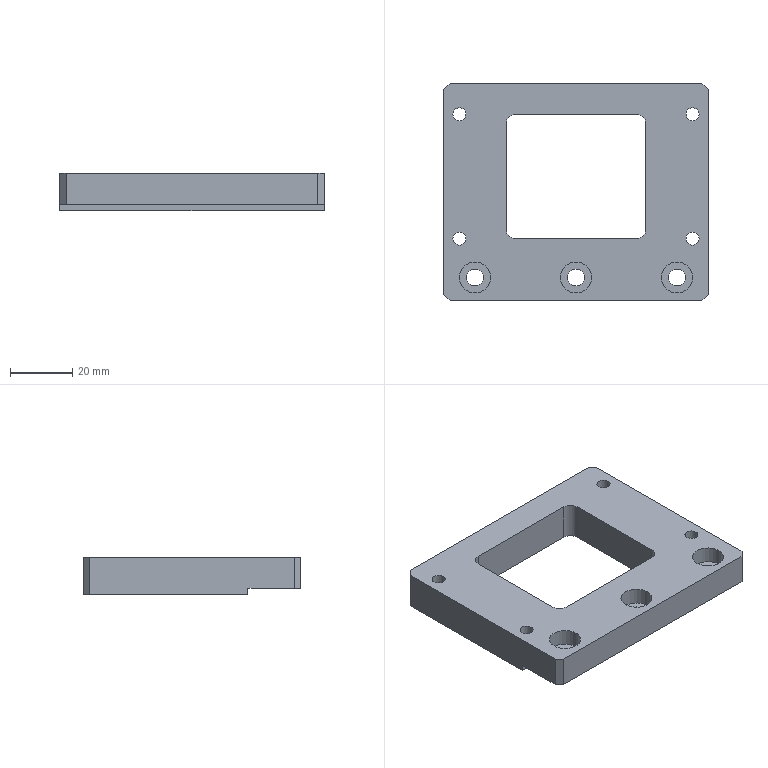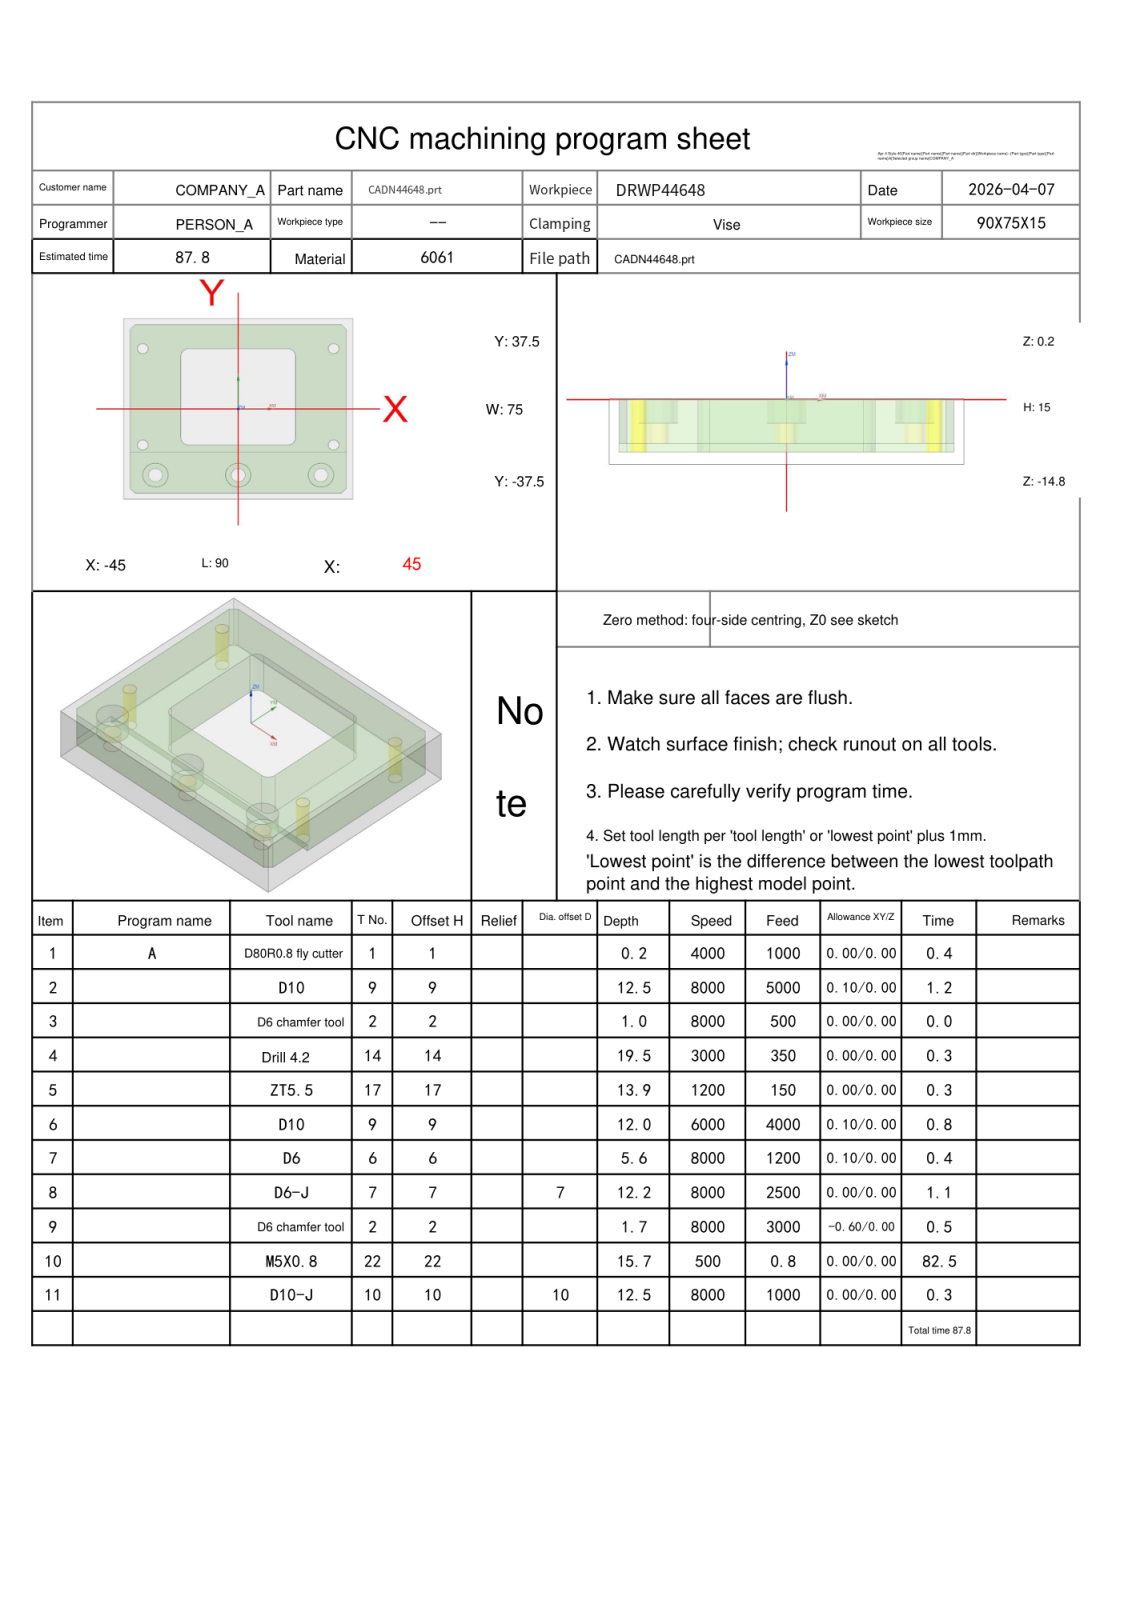NC program | NX | posted by the shop | part box 85 x 70 x 12 mm
Lines 580 to 1629 of 5800:
N8 T07 M06
(D6-J  D=6. R=0. H=07 ce=0.00 di=0.00)
G00 G90 G54 X32.5 Y-27.5 M03 S8000
G43 H07 Z20.
M08
Z0.0
G41 D07
G01 X32.54 Y-27.696 F500.
G03 X33.51 Y-28.49 I.97 J.196
X34.5 Y-27.5 I0.0 J.99
X34.5 Y-27.5 Z-5. I-2. J0.0
X34.253 Y-26.536 Z-5.4 I-2. J0.0
X32.5 Y-25.5 I-1.753 J-.964
X30.5 Y-27.5 I0.0 J-2.
X32.5 Y-29.5 I2. J0.0
X34.5 Y-27.5 I0.0 J2.
X34.253 Y-26.536 I-2. J0.0
X33.385 Y-26.023 I-.868 J-.477
X32.395 Y-27.013 I0.0 J-.99
X32.44 Y-27.309 I.99 J0.0
G01 G40 X32.5 Y-27.5
G00 Z20.
X0.0
Z0.0
G41 D07
G01 X.04 Y-27.696
G03 X1.01 Y-28.49 I.97 J.196
X2. Y-27.5 I0.0 J.99
X2. Y-27.5 Z-5. I-2. J0.0
X1.753 Y-26.536 Z-5.4 I-2. J0.0
X0.0 Y-25.5 I-1.753 J-.964
X-2. Y-27.5 I0.0 J-2.
X0.0 Y-29.5 I2. J0.0
X2. Y-27.5 I0.0 J2.
X1.753 Y-26.536 I-2. J0.0
X.885 Y-26.023 I-.868 J-.477
X-.105 Y-27.013 I0.0 J-.99
X-.06 Y-27.309 I.99 J0.0
G01 G40 X0.0 Y-27.5
G00 Z20.
X-32.5
Z0.0
G41 D07
G01 X-32.46 Y-27.696
G03 X-31.49 Y-28.49 I.97 J.196
X-30.5 Y-27.5 I0.0 J.99
X-30.5 Y-27.5 Z-5. I-2. J0.0
X-30.747 Y-26.536 Z-5.4 I-2. J0.0
X-32.5 Y-25.5 I-1.753 J-.964
X-34.5 Y-27.5 I0.0 J-2.
X-32.5 Y-29.5 I2. J0.0
X-30.5 Y-27.5 I0.0 J2.
X-30.747 Y-26.536 I-2. J0.0
X-31.615 Y-26.023 I-.868 J-.477
X-32.605 Y-27.013 I0.0 J-.99
X-32.56 Y-27.309 I.99 J0.0
G01 G40 X-32.5 Y-27.5
G00 Z20.
G00 G90 X16.684 Y-11.1 M03 S6000
Z20.
Z.6
G01 X16.685 Y-11.11 Z.471 F2000.
X16.69 Y-11.139 Z.355
X16.698 Y-11.183 Z.25
X16.71 Y-11.241 Z.156
X16.726 Y-11.309 Z.072
X16.747 Y-11.385 Z-.001
X16.773 Y-11.466 Z-.065
X16.804 Y-11.55 Z-.12
X16.84 Y-11.634 Z-.166
X16.883 Y-11.715 Z-.205
X16.932 Y-11.791 Z-.236
X16.987 Y-11.859 Z-.261
X17.05 Y-11.917 Z-.279
X17.12 Y-11.961 Z-.291
X17.198 Y-11.99 Z-.298
X17.284 Y-12. Z-.3
X19.5 F2500.
Y-9.784
X19.484 Y-9.711 Z-.301
X19.437 Y-9.657 Z-.304
X19.364 Y-9.619 Z-.308
X19.269 Y-9.598 Z-.313
X19.155 Y-9.59 Z-.32
X19.026 Y-9.596 Z-.328
X18.888 Y-9.613 Z-.338
X18.742 Y-9.642 Z-.347
X18.594 Y-9.679 Z-.358
X18.447 Y-9.725 Z-.369
X18.306 Y-9.778 Z-.381
X18.069 Y-9.89 Z-.404
X17.861 Y-10.023 Z-.427
X17.679 Y-10.179 Z-.45
X17.523 Y-10.361 Z-.473
X17.39 Y-10.569 Z-.496
X17.278 Y-10.806 Z-.519
X17.225 Y-10.947 Z-.531
X17.179 Y-11.094 Z-.542
X17.142 Y-11.242 Z-.553
X17.113 Y-11.388 Z-.562
X17.096 Y-11.526 Z-.572
X17.09 Y-11.655 Z-.58
X17.098 Y-11.769 Z-.587
X17.119 Y-11.864 Z-.592
X17.157 Y-11.937 Z-.596
X17.211 Y-11.984 Z-.599
X17.284 Y-12. Z-.6
X19.5
Y-9.784
X19.484 Y-9.711 Z-.601
X19.437 Y-9.657 Z-.604
X19.364 Y-9.619 Z-.608
X19.269 Y-9.598 Z-.613
X19.155 Y-9.59 Z-.62
X19.026 Y-9.596 Z-.628
X18.888 Y-9.613 Z-.638
X18.742 Y-9.642 Z-.647
X18.594 Y-9.679 Z-.658
X18.447 Y-9.725 Z-.669
X18.306 Y-9.778 Z-.681
X18.069 Y-9.89 Z-.704
X17.861 Y-10.023 Z-.727
X17.679 Y-10.179 Z-.75
X17.523 Y-10.361 Z-.773
X17.39 Y-10.569 Z-.796
X17.278 Y-10.806 Z-.819
X17.225 Y-10.947 Z-.831
X17.179 Y-11.094 Z-.842
X17.142 Y-11.242 Z-.853
X17.113 Y-11.388 Z-.862
X17.096 Y-11.526 Z-.872
X17.09 Y-11.655 Z-.88
X17.098 Y-11.769 Z-.887
X17.119 Y-11.864 Z-.892
X17.157 Y-11.937 Z-.896
X17.211 Y-11.984 Z-.899
X17.284 Y-12. Z-.9
X19.5
Y-9.784
X19.484 Y-9.711 Z-.901
X19.437 Y-9.657 Z-.904
X19.364 Y-9.619 Z-.908
X19.269 Y-9.598 Z-.913
X19.155 Y-9.59 Z-.92
X19.026 Y-9.596 Z-.928
X18.888 Y-9.613 Z-.938
X18.742 Y-9.642 Z-.947
X18.594 Y-9.679 Z-.958
X18.447 Y-9.725 Z-.969
X18.306 Y-9.778 Z-.981
X18.069 Y-9.89 Z-1.004
X17.861 Y-10.023 Z-1.027
X17.679 Y-10.179 Z-1.05
X17.523 Y-10.361 Z-1.073
X17.39 Y-10.569 Z-1.096
X17.278 Y-10.806 Z-1.119
X17.225 Y-10.947 Z-1.131
X17.179 Y-11.094 Z-1.142
X17.142 Y-11.242 Z-1.153
X17.113 Y-11.388 Z-1.162
X17.096 Y-11.526 Z-1.172
X17.09 Y-11.655 Z-1.18
X17.098 Y-11.769 Z-1.187
X17.119 Y-11.864 Z-1.192
X17.157 Y-11.937 Z-1.196
X17.211 Y-11.984 Z-1.199
X17.284 Y-12. Z-1.2
X19.5
Y-9.784
X19.484 Y-9.711 Z-1.201
X19.437 Y-9.657 Z-1.204
X19.364 Y-9.619 Z-1.208
X19.269 Y-9.598 Z-1.213
X19.155 Y-9.59 Z-1.22
X19.026 Y-9.596 Z-1.228
X18.888 Y-9.613 Z-1.238
X18.742 Y-9.642 Z-1.247
X18.594 Y-9.679 Z-1.258
X18.447 Y-9.725 Z-1.269
X18.306 Y-9.778 Z-1.281
X18.069 Y-9.89 Z-1.304
X17.861 Y-10.023 Z-1.327
X17.679 Y-10.179 Z-1.35
X17.523 Y-10.361 Z-1.373
X17.39 Y-10.569 Z-1.396
X17.278 Y-10.806 Z-1.419
X17.225 Y-10.947 Z-1.431
X17.179 Y-11.094 Z-1.442
X17.142 Y-11.242 Z-1.453
X17.113 Y-11.388 Z-1.462
X17.096 Y-11.526 Z-1.472
X17.09 Y-11.655 Z-1.48
X17.098 Y-11.769 Z-1.487
X17.119 Y-11.864 Z-1.492
X17.157 Y-11.937 Z-1.496
X17.211 Y-11.984 Z-1.499
X17.284 Y-12. Z-1.5
X19.5
Y-9.784
X19.484 Y-9.711 Z-1.501
X19.437 Y-9.657 Z-1.504
X19.364 Y-9.619 Z-1.508
X19.269 Y-9.598 Z-1.513
X19.155 Y-9.59 Z-1.52
X19.026 Y-9.596 Z-1.528
X18.888 Y-9.613 Z-1.538
X18.742 Y-9.642 Z-1.547
X18.594 Y-9.679 Z-1.558
X18.447 Y-9.725 Z-1.569
X18.306 Y-9.778 Z-1.581
X18.069 Y-9.89 Z-1.604
X17.861 Y-10.023 Z-1.627
X17.679 Y-10.179 Z-1.65
X17.523 Y-10.361 Z-1.673
X17.39 Y-10.569 Z-1.696
X17.278 Y-10.806 Z-1.719
X17.225 Y-10.947 Z-1.731
X17.179 Y-11.094 Z-1.742
X17.142 Y-11.242 Z-1.753
X17.113 Y-11.388 Z-1.762
X17.096 Y-11.526 Z-1.772
X17.09 Y-11.655 Z-1.78
X17.098 Y-11.769 Z-1.787
X17.119 Y-11.864 Z-1.792
X17.157 Y-11.937 Z-1.796
X17.211 Y-11.984 Z-1.799
X17.284 Y-12. Z-1.8
X19.5
Y-9.784
X19.484 Y-9.711 Z-1.801
X19.437 Y-9.657 Z-1.804
X19.364 Y-9.619 Z-1.808
X19.269 Y-9.598 Z-1.813
X19.155 Y-9.59 Z-1.82
X19.026 Y-9.596 Z-1.828
X18.888 Y-9.613 Z-1.838
X18.742 Y-9.642 Z-1.847
X18.594 Y-9.679 Z-1.858
X18.447 Y-9.725 Z-1.869
X18.306 Y-9.778 Z-1.881
X18.069 Y-9.89 Z-1.904
X17.861 Y-10.023 Z-1.927
X17.679 Y-10.179 Z-1.95
X17.523 Y-10.361 Z-1.973
X17.39 Y-10.569 Z-1.996
X17.278 Y-10.806 Z-2.019
X17.225 Y-10.947 Z-2.031
X17.179 Y-11.094 Z-2.042
X17.142 Y-11.242 Z-2.053
X17.113 Y-11.388 Z-2.062
X17.096 Y-11.526 Z-2.072
X17.09 Y-11.655 Z-2.08
X17.098 Y-11.769 Z-2.087
X17.119 Y-11.864 Z-2.092
X17.157 Y-11.937 Z-2.096
X17.211 Y-11.984 Z-2.099
X17.284 Y-12. Z-2.1
X19.5
Y-9.784
X19.484 Y-9.711 Z-2.101
X19.437 Y-9.657 Z-2.104
X19.364 Y-9.619 Z-2.108
X19.269 Y-9.598 Z-2.113
X19.155 Y-9.59 Z-2.12
X19.026 Y-9.596 Z-2.128
X18.888 Y-9.613 Z-2.138
X18.742 Y-9.642 Z-2.147
X18.594 Y-9.679 Z-2.158
X18.447 Y-9.725 Z-2.169
X18.306 Y-9.778 Z-2.181
X18.069 Y-9.89 Z-2.204
X17.861 Y-10.023 Z-2.227
X17.679 Y-10.179 Z-2.25
X17.523 Y-10.361 Z-2.273
X17.39 Y-10.569 Z-2.296
X17.278 Y-10.806 Z-2.319
X17.225 Y-10.947 Z-2.331
X17.179 Y-11.094 Z-2.342
X17.142 Y-11.242 Z-2.353
X17.113 Y-11.388 Z-2.362
X17.096 Y-11.526 Z-2.372
X17.09 Y-11.655 Z-2.38
X17.098 Y-11.769 Z-2.387
X17.119 Y-11.864 Z-2.392
X17.157 Y-11.937 Z-2.396
X17.211 Y-11.984 Z-2.399
X17.284 Y-12. Z-2.4
X19.5
Y-9.784
X19.484 Y-9.711 Z-2.401
X19.437 Y-9.657 Z-2.404
X19.364 Y-9.619 Z-2.408
X19.269 Y-9.598 Z-2.413
X19.155 Y-9.59 Z-2.42
X19.026 Y-9.596 Z-2.428
X18.888 Y-9.613 Z-2.438
X18.742 Y-9.642 Z-2.447
X18.594 Y-9.679 Z-2.458
X18.447 Y-9.725 Z-2.469
X18.306 Y-9.778 Z-2.481
X18.069 Y-9.89 Z-2.504
X17.861 Y-10.023 Z-2.527
X17.679 Y-10.179 Z-2.55
X17.523 Y-10.361 Z-2.573
X17.39 Y-10.569 Z-2.596
X17.278 Y-10.806 Z-2.619
X17.225 Y-10.947 Z-2.631
X17.179 Y-11.094 Z-2.642
X17.142 Y-11.242 Z-2.653
X17.113 Y-11.388 Z-2.662
X17.096 Y-11.526 Z-2.672
X17.09 Y-11.655 Z-2.68
X17.098 Y-11.769 Z-2.687
X17.119 Y-11.864 Z-2.692
X17.157 Y-11.937 Z-2.696
X17.211 Y-11.984 Z-2.699
X17.284 Y-12. Z-2.7
X19.5
Y-9.784
X19.484 Y-9.711 Z-2.701
X19.437 Y-9.657 Z-2.704
X19.364 Y-9.619 Z-2.708
X19.269 Y-9.598 Z-2.713
X19.155 Y-9.59 Z-2.72
X19.026 Y-9.596 Z-2.728
X18.888 Y-9.613 Z-2.738
X18.742 Y-9.642 Z-2.747
X18.594 Y-9.679 Z-2.758
X18.447 Y-9.725 Z-2.769
X18.306 Y-9.778 Z-2.781
X18.069 Y-9.89 Z-2.804
X17.861 Y-10.023 Z-2.827
X17.679 Y-10.179 Z-2.85
X17.523 Y-10.361 Z-2.873
X17.39 Y-10.569 Z-2.896
X17.278 Y-10.806 Z-2.919
X17.225 Y-10.947 Z-2.931
X17.179 Y-11.094 Z-2.942
X17.142 Y-11.242 Z-2.953
X17.113 Y-11.388 Z-2.962
X17.096 Y-11.526 Z-2.972
X17.09 Y-11.655 Z-2.98
X17.098 Y-11.769 Z-2.987
X17.119 Y-11.864 Z-2.992
X17.157 Y-11.937 Z-2.996
X17.211 Y-11.984 Z-2.999
X17.284 Y-12. Z-3.
X19.5
Y-9.784
X19.484 Y-9.711 Z-3.001
X19.437 Y-9.657 Z-3.004
X19.364 Y-9.619 Z-3.008
X19.269 Y-9.598 Z-3.013
X19.155 Y-9.59 Z-3.02
X19.026 Y-9.596 Z-3.028
X18.888 Y-9.613 Z-3.038
X18.742 Y-9.642 Z-3.047
X18.594 Y-9.679 Z-3.058
X18.447 Y-9.725 Z-3.069
X18.306 Y-9.778 Z-3.081
X18.069 Y-9.89 Z-3.104
X17.861 Y-10.023 Z-3.127
X17.679 Y-10.179 Z-3.15
X17.523 Y-10.361 Z-3.173
X17.39 Y-10.569 Z-3.196
X17.278 Y-10.806 Z-3.219
X17.225 Y-10.947 Z-3.231
X17.179 Y-11.094 Z-3.242
X17.142 Y-11.242 Z-3.253
X17.113 Y-11.388 Z-3.262
X17.096 Y-11.526 Z-3.272
X17.09 Y-11.655 Z-3.28
X17.098 Y-11.769 Z-3.287
X17.119 Y-11.864 Z-3.292
X17.157 Y-11.937 Z-3.296
X17.211 Y-11.984 Z-3.299
X17.284 Y-12. Z-3.3
X19.5
Y-9.784
X19.484 Y-9.711 Z-3.301
X19.437 Y-9.657 Z-3.304
X19.364 Y-9.619 Z-3.308
X19.269 Y-9.598 Z-3.313
X19.155 Y-9.59 Z-3.32
X19.026 Y-9.596 Z-3.328
X18.888 Y-9.613 Z-3.338
X18.742 Y-9.642 Z-3.347
X18.594 Y-9.679 Z-3.358
X18.447 Y-9.725 Z-3.369
X18.306 Y-9.778 Z-3.381
X18.069 Y-9.89 Z-3.404
X17.861 Y-10.023 Z-3.427
X17.679 Y-10.179 Z-3.45
X17.523 Y-10.361 Z-3.473
X17.39 Y-10.569 Z-3.496
X17.278 Y-10.806 Z-3.519
X17.225 Y-10.947 Z-3.531
X17.179 Y-11.094 Z-3.542
X17.142 Y-11.242 Z-3.553
X17.113 Y-11.388 Z-3.562
X17.096 Y-11.526 Z-3.572
X17.09 Y-11.655 Z-3.58
X17.098 Y-11.769 Z-3.587
X17.119 Y-11.864 Z-3.592
X17.157 Y-11.937 Z-3.596
X17.211 Y-11.984 Z-3.599
X17.284 Y-12. Z-3.6
X19.5
Y-9.784
X19.484 Y-9.711 Z-3.601
X19.437 Y-9.657 Z-3.604
X19.364 Y-9.619 Z-3.608
X19.269 Y-9.598 Z-3.613
X19.155 Y-9.59 Z-3.62
X19.026 Y-9.596 Z-3.628
X18.888 Y-9.613 Z-3.638
X18.742 Y-9.642 Z-3.647
X18.594 Y-9.679 Z-3.658
X18.447 Y-9.725 Z-3.669
X18.306 Y-9.778 Z-3.681
X18.069 Y-9.89 Z-3.704
X17.861 Y-10.023 Z-3.727
X17.679 Y-10.179 Z-3.75
X17.523 Y-10.361 Z-3.773
X17.39 Y-10.569 Z-3.796
X17.278 Y-10.806 Z-3.819
X17.225 Y-10.947 Z-3.831
X17.179 Y-11.094 Z-3.842
X17.142 Y-11.242 Z-3.853
X17.113 Y-11.388 Z-3.862
X17.096 Y-11.526 Z-3.872
X17.09 Y-11.655 Z-3.88
X17.098 Y-11.769 Z-3.887
X17.119 Y-11.864 Z-3.892
X17.157 Y-11.937 Z-3.896
X17.211 Y-11.984 Z-3.899
X17.284 Y-12. Z-3.9
X19.5
Y-9.784
X19.484 Y-9.711 Z-3.901
X19.437 Y-9.657 Z-3.904
X19.364 Y-9.619 Z-3.908
X19.269 Y-9.598 Z-3.913
X19.155 Y-9.59 Z-3.92
X19.026 Y-9.596 Z-3.928
X18.888 Y-9.613 Z-3.938
X18.742 Y-9.642 Z-3.947
X18.594 Y-9.679 Z-3.958
X18.447 Y-9.725 Z-3.969
X18.306 Y-9.778 Z-3.981
X18.069 Y-9.89 Z-4.004
X17.861 Y-10.023 Z-4.027
X17.679 Y-10.179 Z-4.05
X17.523 Y-10.361 Z-4.073
X17.39 Y-10.569 Z-4.096
X17.278 Y-10.806 Z-4.119
X17.225 Y-10.947 Z-4.131
X17.179 Y-11.094 Z-4.142
X17.142 Y-11.242 Z-4.153
X17.113 Y-11.388 Z-4.162
X17.096 Y-11.526 Z-4.172
X17.09 Y-11.655 Z-4.18
X17.098 Y-11.769 Z-4.187
X17.119 Y-11.864 Z-4.192
X17.157 Y-11.937 Z-4.196
X17.211 Y-11.984 Z-4.199
X17.284 Y-12. Z-4.2
X19.5
Y-9.784
X19.484 Y-9.711 Z-4.201
X19.437 Y-9.657 Z-4.204
X19.364 Y-9.619 Z-4.208
X19.269 Y-9.598 Z-4.213
X19.155 Y-9.59 Z-4.22
X19.026 Y-9.596 Z-4.228
X18.888 Y-9.613 Z-4.238
X18.742 Y-9.642 Z-4.247
X18.594 Y-9.679 Z-4.258
X18.447 Y-9.725 Z-4.269
X18.306 Y-9.778 Z-4.281
X18.069 Y-9.89 Z-4.304
X17.861 Y-10.023 Z-4.327
X17.679 Y-10.179 Z-4.35
X17.523 Y-10.361 Z-4.373
X17.39 Y-10.569 Z-4.396
X17.278 Y-10.806 Z-4.419
X17.225 Y-10.947 Z-4.431
X17.179 Y-11.094 Z-4.442
X17.142 Y-11.242 Z-4.453
X17.113 Y-11.388 Z-4.462
X17.096 Y-11.526 Z-4.472
X17.09 Y-11.655 Z-4.48
X17.098 Y-11.769 Z-4.487
X17.119 Y-11.864 Z-4.492
X17.157 Y-11.937 Z-4.496
X17.211 Y-11.984 Z-4.499
X17.284 Y-12. Z-4.5
X19.5
Y-9.784
X19.484 Y-9.711 Z-4.501
X19.437 Y-9.657 Z-4.504
X19.364 Y-9.619 Z-4.508
X19.269 Y-9.598 Z-4.513
X19.155 Y-9.59 Z-4.52
X19.026 Y-9.596 Z-4.528
X18.888 Y-9.613 Z-4.538
X18.742 Y-9.642 Z-4.547
X18.594 Y-9.679 Z-4.558
X18.447 Y-9.725 Z-4.569
X18.306 Y-9.778 Z-4.581
X18.069 Y-9.89 Z-4.604
X17.861 Y-10.023 Z-4.627
X17.679 Y-10.179 Z-4.65
X17.523 Y-10.361 Z-4.673
X17.39 Y-10.569 Z-4.696
X17.278 Y-10.806 Z-4.719
X17.225 Y-10.947 Z-4.731
X17.179 Y-11.094 Z-4.742
X17.142 Y-11.242 Z-4.753
X17.113 Y-11.388 Z-4.762
X17.096 Y-11.526 Z-4.772
X17.09 Y-11.655 Z-4.78
X17.098 Y-11.769 Z-4.787
X17.119 Y-11.864 Z-4.792
X17.157 Y-11.937 Z-4.796
X17.211 Y-11.984 Z-4.799
X17.284 Y-12. Z-4.8
X19.5
Y-9.784
X19.484 Y-9.711 Z-4.801
X19.437 Y-9.657 Z-4.804
X19.364 Y-9.619 Z-4.808
X19.269 Y-9.598 Z-4.813
X19.155 Y-9.59 Z-4.82
X19.026 Y-9.596 Z-4.828
X18.888 Y-9.613 Z-4.838
X18.742 Y-9.642 Z-4.847
X18.594 Y-9.679 Z-4.858
X18.447 Y-9.725 Z-4.869
X18.306 Y-9.778 Z-4.881
X18.069 Y-9.89 Z-4.904
X17.861 Y-10.023 Z-4.927
X17.679 Y-10.179 Z-4.95
X17.523 Y-10.361 Z-4.973
X17.39 Y-10.569 Z-4.996
X17.278 Y-10.806 Z-5.019
X17.225 Y-10.947 Z-5.031
X17.179 Y-11.094 Z-5.042
X17.142 Y-11.242 Z-5.053
X17.113 Y-11.388 Z-5.062
X17.096 Y-11.526 Z-5.072
X17.09 Y-11.655 Z-5.08
X17.098 Y-11.769 Z-5.087
X17.119 Y-11.864 Z-5.092
X17.157 Y-11.937 Z-5.096
X17.211 Y-11.984 Z-5.099
X17.284 Y-12. Z-5.1
X19.5
Y-9.784
X19.484 Y-9.711 Z-5.101
X19.437 Y-9.657 Z-5.104
X19.364 Y-9.619 Z-5.108
X19.269 Y-9.598 Z-5.113
X19.155 Y-9.59 Z-5.12
X19.026 Y-9.596 Z-5.128
X18.888 Y-9.613 Z-5.138
X18.742 Y-9.642 Z-5.147
X18.594 Y-9.679 Z-5.158
X18.447 Y-9.725 Z-5.169
X18.306 Y-9.778 Z-5.181
X18.069 Y-9.89 Z-5.204
X17.861 Y-10.023 Z-5.227
X17.679 Y-10.179 Z-5.25
X17.523 Y-10.361 Z-5.273
X17.39 Y-10.569 Z-5.296
X17.278 Y-10.806 Z-5.319
X17.225 Y-10.947 Z-5.331
X17.179 Y-11.094 Z-5.342
X17.142 Y-11.242 Z-5.353
X17.113 Y-11.388 Z-5.362
X17.096 Y-11.526 Z-5.372
X17.09 Y-11.655 Z-5.38
X17.098 Y-11.769 Z-5.387
X17.119 Y-11.864 Z-5.392
X17.157 Y-11.937 Z-5.396
X17.211 Y-11.984 Z-5.399
X17.284 Y-12. Z-5.4
X19.5
Y-9.784
X19.484 Y-9.711 Z-5.401
X19.437 Y-9.657 Z-5.404
X19.364 Y-9.619 Z-5.408
X19.269 Y-9.598 Z-5.413
X19.155 Y-9.59 Z-5.42
X19.026 Y-9.596 Z-5.428
X18.888 Y-9.613 Z-5.438
X18.742 Y-9.642 Z-5.447
X18.594 Y-9.679 Z-5.458
X18.447 Y-9.725 Z-5.469
X18.306 Y-9.778 Z-5.481
X18.069 Y-9.89 Z-5.504
X17.861 Y-10.023 Z-5.527
X17.679 Y-10.179 Z-5.55
X17.523 Y-10.361 Z-5.573
X17.39 Y-10.569 Z-5.596
X17.278 Y-10.806 Z-5.619
X17.225 Y-10.947 Z-5.631
X17.179 Y-11.094 Z-5.642
X17.142 Y-11.242 Z-5.653
X17.113 Y-11.388 Z-5.662
X17.096 Y-11.526 Z-5.672
X17.09 Y-11.655 Z-5.68
X17.098 Y-11.769 Z-5.687
X17.119 Y-11.864 Z-5.692
X17.157 Y-11.937 Z-5.696
X17.211 Y-11.984 Z-5.699
X17.284 Y-12. Z-5.7
X19.5
Y-9.784
X19.484 Y-9.711 Z-5.701
X19.437 Y-9.657 Z-5.704
X19.364 Y-9.619 Z-5.708
X19.269 Y-9.598 Z-5.713
X19.155 Y-9.59 Z-5.72
X19.026 Y-9.596 Z-5.728
X18.888 Y-9.613 Z-5.738
X18.742 Y-9.642 Z-5.747
X18.594 Y-9.679 Z-5.758
X18.447 Y-9.725 Z-5.769
X18.306 Y-9.778 Z-5.781
X18.069 Y-9.89 Z-5.804
X17.861 Y-10.023 Z-5.827
X17.679 Y-10.179 Z-5.85
X17.523 Y-10.361 Z-5.873
X17.39 Y-10.569 Z-5.896
X17.278 Y-10.806 Z-5.919
X17.225 Y-10.947 Z-5.931
X17.179 Y-11.094 Z-5.942
X17.142 Y-11.242 Z-5.953
X17.113 Y-11.388 Z-5.962
X17.096 Y-11.526 Z-5.972
X17.09 Y-11.655 Z-5.98
X17.098 Y-11.769 Z-5.987
X17.119 Y-11.864 Z-5.992
X17.157 Y-11.937 Z-5.996
X17.211 Y-11.984 Z-5.999
X17.284 Y-12. Z-6.
X19.5
Y-9.784
X19.484 Y-9.711 Z-6.001
X19.437 Y-9.657 Z-6.004
X19.364 Y-9.619 Z-6.008
X19.269 Y-9.598 Z-6.013
X19.155 Y-9.59 Z-6.02
X19.026 Y-9.596 Z-6.028
X18.888 Y-9.613 Z-6.038
X18.742 Y-9.642 Z-6.047
X18.594 Y-9.679 Z-6.058
X18.447 Y-9.725 Z-6.069
X18.306 Y-9.778 Z-6.081
X18.069 Y-9.89 Z-6.104
X17.861 Y-10.023 Z-6.127
X17.679 Y-10.179 Z-6.15
X17.523 Y-10.361 Z-6.173
X17.39 Y-10.569 Z-6.196
X17.278 Y-10.806 Z-6.219
X17.225 Y-10.947 Z-6.231
X17.179 Y-11.094 Z-6.242
X17.142 Y-11.242 Z-6.253
X17.113 Y-11.388 Z-6.262
X17.096 Y-11.526 Z-6.272
X17.09 Y-11.655 Z-6.28
X17.098 Y-11.769 Z-6.287
X17.119 Y-11.864 Z-6.292
X17.157 Y-11.937 Z-6.296
X17.211 Y-11.984 Z-6.299
X17.284 Y-12. Z-6.3
X19.5
Y-9.784
X19.484 Y-9.711 Z-6.301
X19.437 Y-9.657 Z-6.304
X19.364 Y-9.619 Z-6.308
X19.269 Y-9.598 Z-6.313
X19.155 Y-9.59 Z-6.32
X19.026 Y-9.596 Z-6.328
X18.888 Y-9.613 Z-6.338
X18.742 Y-9.642 Z-6.347
X18.594 Y-9.679 Z-6.358
X18.447 Y-9.725 Z-6.369
X18.306 Y-9.778 Z-6.381
X18.069 Y-9.89 Z-6.404
X17.861 Y-10.023 Z-6.427
X17.679 Y-10.179 Z-6.45
X17.523 Y-10.361 Z-6.473
X17.39 Y-10.569 Z-6.496
X17.278 Y-10.806 Z-6.519
X17.225 Y-10.947 Z-6.531
X17.179 Y-11.094 Z-6.542
X17.142 Y-11.242 Z-6.553
X17.113 Y-11.388 Z-6.562
X17.096 Y-11.526 Z-6.572
X17.09 Y-11.655 Z-6.58
X17.098 Y-11.769 Z-6.587
X17.119 Y-11.864 Z-6.592
X17.157 Y-11.937 Z-6.596
X17.211 Y-11.984 Z-6.599
X17.284 Y-12. Z-6.6
X19.5
Y-9.784
X19.484 Y-9.711 Z-6.601
X19.437 Y-9.657 Z-6.604
X19.364 Y-9.619 Z-6.608
X19.269 Y-9.598 Z-6.613
X19.155 Y-9.59 Z-6.62
X19.026 Y-9.596 Z-6.628
X18.888 Y-9.613 Z-6.638
X18.742 Y-9.642 Z-6.647
X18.594 Y-9.679 Z-6.658
X18.447 Y-9.725 Z-6.669
X18.306 Y-9.778 Z-6.681
X18.069 Y-9.89 Z-6.704
X17.861 Y-10.023 Z-6.727
X17.679 Y-10.179 Z-6.75
X17.523 Y-10.361 Z-6.773
X17.39 Y-10.569 Z-6.796
X17.278 Y-10.806 Z-6.819
X17.225 Y-10.947 Z-6.831
X17.179 Y-11.094 Z-6.842
X17.142 Y-11.242 Z-6.853
X17.113 Y-11.388 Z-6.862
X17.096 Y-11.526 Z-6.872
X17.09 Y-11.655 Z-6.88
X17.098 Y-11.769 Z-6.887
X17.119 Y-11.864 Z-6.892
X17.157 Y-11.937 Z-6.896
X17.211 Y-11.984 Z-6.899
X17.284 Y-12. Z-6.9
X19.5
Y-9.784
X19.484 Y-9.711 Z-6.901
X19.437 Y-9.657 Z-6.904
X19.364 Y-9.619 Z-6.908
X19.269 Y-9.598 Z-6.913
X19.155 Y-9.59 Z-6.92
X19.026 Y-9.596 Z-6.928
X18.888 Y-9.613 Z-6.938
X18.742 Y-9.642 Z-6.947
X18.594 Y-9.679 Z-6.958
X18.447 Y-9.725 Z-6.969
X18.306 Y-9.778 Z-6.981
X18.069 Y-9.89 Z-7.004
X17.861 Y-10.023 Z-7.027
X17.679 Y-10.179 Z-7.05
X17.523 Y-10.361 Z-7.073
X17.39 Y-10.569 Z-7.096
X17.278 Y-10.806 Z-7.119
X17.225 Y-10.947 Z-7.131
X17.179 Y-11.094 Z-7.142
X17.142 Y-11.242 Z-7.153
X17.113 Y-11.388 Z-7.162
X17.096 Y-11.526 Z-7.172
X17.09 Y-11.655 Z-7.18
X17.098 Y-11.769 Z-7.187
X17.119 Y-11.864 Z-7.192
X17.157 Y-11.937 Z-7.196
X17.211 Y-11.984 Z-7.199
X17.284 Y-12. Z-7.2
X19.5
Y-9.784
X19.484 Y-9.711 Z-7.201
X19.437 Y-9.657 Z-7.204
X19.364 Y-9.619 Z-7.208
X19.269 Y-9.598 Z-7.213
X19.155 Y-9.59 Z-7.22
X19.026 Y-9.596 Z-7.228
X18.888 Y-9.613 Z-7.238
X18.742 Y-9.642 Z-7.247
X18.594 Y-9.679 Z-7.258
X18.447 Y-9.725 Z-7.269
X18.306 Y-9.778 Z-7.281
X18.069 Y-9.89 Z-7.304
X17.861 Y-10.023 Z-7.327
X17.679 Y-10.179 Z-7.35
X17.523 Y-10.361 Z-7.373
X17.39 Y-10.569 Z-7.396
X17.278 Y-10.806 Z-7.419
X17.225 Y-10.947 Z-7.431
X17.179 Y-11.094 Z-7.442
X17.142 Y-11.242 Z-7.453
X17.113 Y-11.388 Z-7.462
X17.096 Y-11.526 Z-7.472
X17.09 Y-11.655 Z-7.48
X17.098 Y-11.769 Z-7.487
X17.119 Y-11.864 Z-7.492
X17.157 Y-11.937 Z-7.496
X17.211 Y-11.984 Z-7.499
X17.284 Y-12. Z-7.5
X19.5
Y-9.784
X19.484 Y-9.711 Z-7.501
X19.437 Y-9.657 Z-7.504
X19.364 Y-9.619 Z-7.508
X19.269 Y-9.598 Z-7.513
X19.155 Y-9.59 Z-7.52
X19.026 Y-9.596 Z-7.528
X18.888 Y-9.613 Z-7.538
X18.742 Y-9.642 Z-7.547
X18.594 Y-9.679 Z-7.558
X18.447 Y-9.725 Z-7.569
X18.306 Y-9.778 Z-7.581
X18.069 Y-9.89 Z-7.604
X17.861 Y-10.023 Z-7.627
X17.679 Y-10.179 Z-7.65
X17.523 Y-10.361 Z-7.673
X17.39 Y-10.569 Z-7.696
X17.278 Y-10.806 Z-7.719
X17.225 Y-10.947 Z-7.731
X17.179 Y-11.094 Z-7.742
X17.142 Y-11.242 Z-7.753
X17.113 Y-11.388 Z-7.762
X17.096 Y-11.526 Z-7.772
X17.09 Y-11.655 Z-7.78
X17.098 Y-11.769 Z-7.787
X17.119 Y-11.864 Z-7.792
X17.157 Y-11.937 Z-7.796
X17.211 Y-11.984 Z-7.799
X17.284 Y-12. Z-7.8
X19.5
Y-9.784
X19.484 Y-9.711 Z-7.801
X19.437 Y-9.657 Z-7.804
X19.364 Y-9.619 Z-7.808
X19.269 Y-9.598 Z-7.813
X19.155 Y-9.59 Z-7.82
X19.026 Y-9.596 Z-7.828
X18.888 Y-9.613 Z-7.838
X18.742 Y-9.642 Z-7.847
X18.594 Y-9.679 Z-7.858
X18.447 Y-9.725 Z-7.869
X18.306 Y-9.778 Z-7.881
X18.069 Y-9.89 Z-7.904
X17.861 Y-10.023 Z-7.927
X17.679 Y-10.179 Z-7.95
X17.523 Y-10.361 Z-7.973
X17.39 Y-10.569 Z-7.996
X17.278 Y-10.806 Z-8.019
X17.225 Y-10.947 Z-8.031
X17.179 Y-11.094 Z-8.042
X17.142 Y-11.242 Z-8.053
X17.113 Y-11.388 Z-8.062
X17.096 Y-11.526 Z-8.072
X17.09 Y-11.655 Z-8.08
X17.098 Y-11.769 Z-8.087
X17.119 Y-11.864 Z-8.092
X17.157 Y-11.937 Z-8.096
X17.211 Y-11.984 Z-8.099
X17.284 Y-12. Z-8.1
X19.5
Y-9.784
X19.484 Y-9.711 Z-8.101
X19.437 Y-9.657 Z-8.104
X19.364 Y-9.619 Z-8.108
X19.269 Y-9.598 Z-8.113
X19.155 Y-9.59 Z-8.12
X19.026 Y-9.596 Z-8.128
X18.888 Y-9.613 Z-8.138
X18.742 Y-9.642 Z-8.147
X18.594 Y-9.679 Z-8.158
X18.447 Y-9.725 Z-8.169
X18.306 Y-9.778 Z-8.181
X18.069 Y-9.89 Z-8.204
X17.861 Y-10.023 Z-8.227
X17.679 Y-10.179 Z-8.25
X17.523 Y-10.361 Z-8.273
X17.39 Y-10.569 Z-8.296
X17.278 Y-10.806 Z-8.319
X17.225 Y-10.947 Z-8.331
X17.179 Y-11.094 Z-8.342
X17.142 Y-11.242 Z-8.353
X17.113 Y-11.388 Z-8.362
X17.096 Y-11.526 Z-8.372
X17.09 Y-11.655 Z-8.38
X17.098 Y-11.769 Z-8.387
X17.119 Y-11.864 Z-8.392
X17.157 Y-11.937 Z-8.396
X17.211 Y-11.984 Z-8.399
X17.284 Y-12. Z-8.4
X19.5
Y-9.784
X19.484 Y-9.711 Z-8.401
X19.437 Y-9.657 Z-8.404
X19.364 Y-9.619 Z-8.408
X19.269 Y-9.598 Z-8.413
X19.155 Y-9.59 Z-8.42
X19.026 Y-9.596 Z-8.428
X18.888 Y-9.613 Z-8.438
X18.742 Y-9.642 Z-8.447
X18.594 Y-9.679 Z-8.458
X18.447 Y-9.725 Z-8.469
X18.306 Y-9.778 Z-8.481
X18.069 Y-9.89 Z-8.504
X17.861 Y-10.023 Z-8.527
X17.679 Y-10.179 Z-8.55
X17.523 Y-10.361 Z-8.573
X17.39 Y-10.569 Z-8.596
X17.278 Y-10.806 Z-8.619
X17.225 Y-10.947 Z-8.631
X17.179 Y-11.094 Z-8.642
X17.142 Y-11.242 Z-8.653
X17.113 Y-11.388 Z-8.662
X17.096 Y-11.526 Z-8.672
X17.09 Y-11.655 Z-8.68
X17.098 Y-11.769 Z-8.687
X17.119 Y-11.864 Z-8.692
X17.157 Y-11.937 Z-8.696
X17.211 Y-11.984 Z-8.699
X17.284 Y-12. Z-8.7
X19.5
Y-9.784
X19.484 Y-9.711 Z-8.701
X19.437 Y-9.657 Z-8.704
X19.364 Y-9.619 Z-8.708
X19.269 Y-9.598 Z-8.713
X19.155 Y-9.59 Z-8.72
X19.026 Y-9.596 Z-8.728
X18.888 Y-9.613 Z-8.738
X18.742 Y-9.642 Z-8.747
X18.594 Y-9.679 Z-8.758
X18.447 Y-9.725 Z-8.769
X18.306 Y-9.778 Z-8.781
X18.069 Y-9.89 Z-8.804
X17.861 Y-10.023 Z-8.827
X17.679 Y-10.179 Z-8.85
X17.523 Y-10.361 Z-8.873
X17.39 Y-10.569 Z-8.896
X17.278 Y-10.806 Z-8.919
X17.225 Y-10.947 Z-8.931
X17.179 Y-11.094 Z-8.942
X17.142 Y-11.242 Z-8.953
X17.113 Y-11.388 Z-8.962
X17.096 Y-11.526 Z-8.972
X17.09 Y-11.655 Z-8.98
X17.098 Y-11.769 Z-8.987
X17.119 Y-11.864 Z-8.992
X17.157 Y-11.937 Z-8.996
X17.211 Y-11.984 Z-8.999
X17.284 Y-12. Z-9.
X19.5
Y-9.784
X19.484 Y-9.711 Z-9.001
X19.437 Y-9.657 Z-9.004
X19.364 Y-9.619 Z-9.008
X19.269 Y-9.598 Z-9.013
X19.155 Y-9.59 Z-9.02
X19.026 Y-9.596 Z-9.028
X18.888 Y-9.613 Z-9.038
X18.742 Y-9.642 Z-9.047
X18.594 Y-9.679 Z-9.058
X18.447 Y-9.725 Z-9.069
X18.306 Y-9.778 Z-9.081
X18.069 Y-9.89 Z-9.104
X17.861 Y-10.023 Z-9.127
X17.679 Y-10.179 Z-9.15
X17.523 Y-10.361 Z-9.173
X17.39 Y-10.569 Z-9.196
X17.278 Y-10.806 Z-9.219
X17.225 Y-10.947 Z-9.231
X17.179 Y-11.094 Z-9.242
X17.142 Y-11.242 Z-9.253
X17.113 Y-11.388 Z-9.262
X17.096 Y-11.526 Z-9.272
X17.09 Y-11.655 Z-9.28
X17.098 Y-11.769 Z-9.287
X17.119 Y-11.864 Z-9.292
X17.157 Y-11.937 Z-9.296
X17.211 Y-11.984 Z-9.299
X17.284 Y-12. Z-9.3
X19.5
Y-9.784
X19.484 Y-9.711 Z-9.301
X19.437 Y-9.657 Z-9.304
X19.364 Y-9.619 Z-9.308
X19.269 Y-9.598 Z-9.313
X19.155 Y-9.59 Z-9.32
X19.026 Y-9.596 Z-9.328
X18.888 Y-9.613 Z-9.338
X18.742 Y-9.642 Z-9.347
X18.594 Y-9.679 Z-9.358
X18.447 Y-9.725 Z-9.369
X18.306 Y-9.778 Z-9.381
X18.069 Y-9.89 Z-9.404
X17.861 Y-10.023 Z-9.427
X17.679 Y-10.179 Z-9.45
X17.523 Y-10.361 Z-9.473
X17.39 Y-10.569 Z-9.496
X17.278 Y-10.806 Z-9.519
X17.225 Y-10.947 Z-9.531
X17.179 Y-11.094 Z-9.542
X17.142 Y-11.242 Z-9.553
X17.113 Y-11.388 Z-9.562
X17.096 Y-11.526 Z-9.572
X17.09 Y-11.655 Z-9.58
X17.098 Y-11.769 Z-9.587
X17.119 Y-11.864 Z-9.592
X17.157 Y-11.937 Z-9.596
X17.211 Y-11.984 Z-9.599
X17.284 Y-12. Z-9.6
X19.5
Y-9.784
X19.484 Y-9.711 Z-9.601
X19.437 Y-9.657 Z-9.604
X19.364 Y-9.619 Z-9.608
X19.269 Y-9.598 Z-9.613
X19.155 Y-9.59 Z-9.62
X19.026 Y-9.596 Z-9.628
X18.888 Y-9.613 Z-9.638
X18.742 Y-9.642 Z-9.647
X18.594 Y-9.679 Z-9.658
X18.447 Y-9.725 Z-9.669
X18.306 Y-9.778 Z-9.681
X18.069 Y-9.89 Z-9.704
X17.861 Y-10.023 Z-9.727
X17.679 Y-10.179 Z-9.75
X17.523 Y-10.361 Z-9.773
X17.39 Y-10.569 Z-9.796
X17.278 Y-10.806 Z-9.819
X17.225 Y-10.947 Z-9.831
X17.179 Y-11.094 Z-9.842
X17.142 Y-11.242 Z-9.853
X17.113 Y-11.388 Z-9.862
X17.096 Y-11.526 Z-9.872
X17.09 Y-11.655 Z-9.88
X17.098 Y-11.769 Z-9.887
X17.119 Y-11.864 Z-9.892
X17.157 Y-11.937 Z-9.896
X17.211 Y-11.984 Z-9.899
X17.284 Y-12. Z-9.9
X19.5
Y-9.784
X19.484 Y-9.711 Z-9.901
X19.437 Y-9.657 Z-9.904
X19.364 Y-9.619 Z-9.908
X19.269 Y-9.598 Z-9.913
X19.155 Y-9.59 Z-9.92
X19.026 Y-9.596 Z-9.928
X18.888 Y-9.613 Z-9.938
X18.742 Y-9.642 Z-9.947
X18.594 Y-9.679 Z-9.958
X18.447 Y-9.725 Z-9.969
X18.306 Y-9.778 Z-9.981